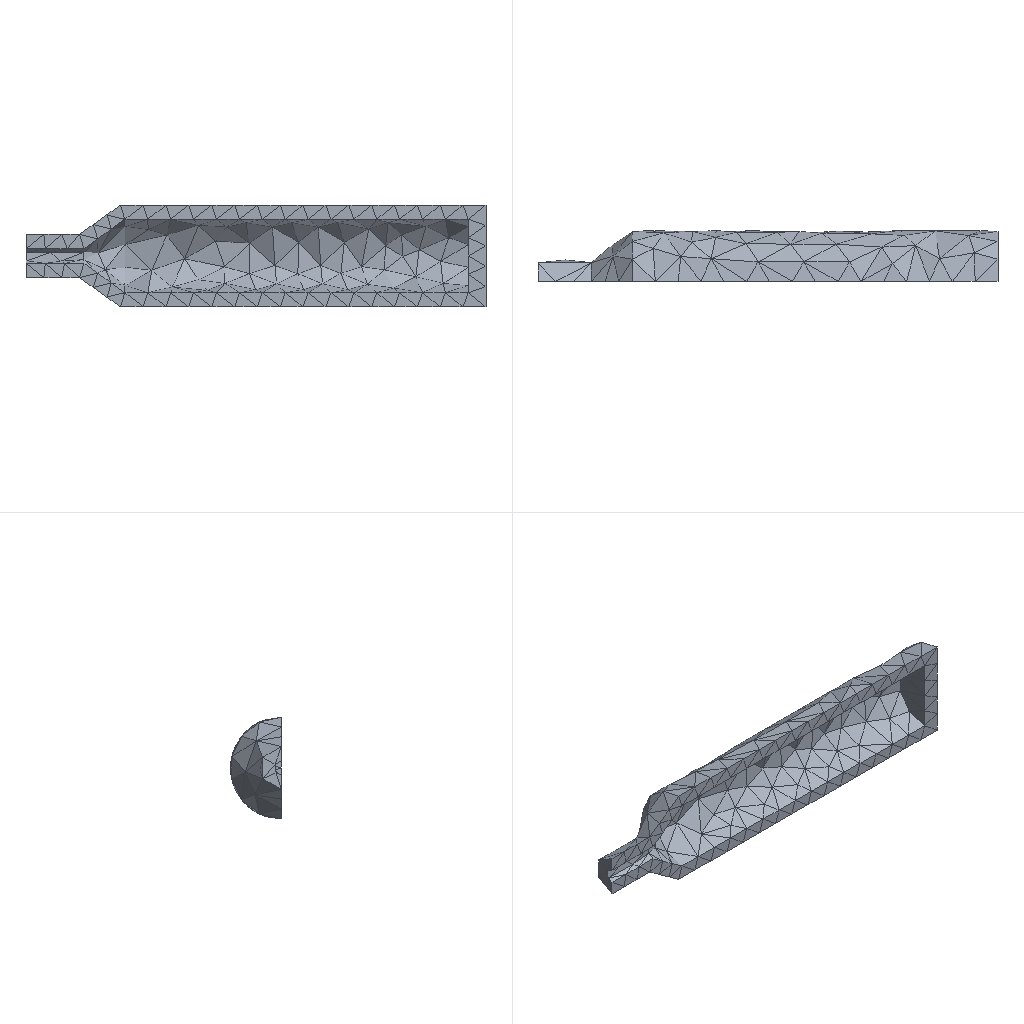Simulation study | ansys workbench
Ansys APDL input file, long lists of numbers shortened:
/batch
/config,noeldb,1     ! force off writing results to database
*get,_wallstrt,active,,time,wall
! ANSYS input file written by Workbench version 2022 R1
! File used for geometry attach:
/title,____--____ (B5)
! ****** Begin Custom Load Command Snippet ******
/COM, ACT Extensions:
/COM,     LSDYNA, 2021.1
/COM,
! ****** End   Custom Load Command Snippet ******
*DIM,_wb_ProjectScratch_dir,string,248
_wb_ProjectScratch_dir(1) = ''
*DIM,_wb_SolverFiles_dir,string,248
_wb_SolverFiles_dir(1) = ''
*DIM,_wb_userfiles_dir,string,248
_wb_userfiles_dir(1) = ''
/com,--- Data in consistent NMM units. See Solving Units in the help system for more information.
/units,MPA
/nopr
/wb,file,start              !  signify a WB generated input file
/prep7
! Turn off shape checking because checks already performed inside WB mesher.
! See help system for more information.
SHPP,OFF,,NOWARN
/nolist
etcon,set             ! allow ANSYS to choose best KEYOP's for 180x elements, resets any applicable keyopt to MAPDL defaults
/com,*********** Nodes for the whole assembly ***********
nblock,3,,1436
(1i9,3e20.9e3)
        1     1.304000000E+03     0.000000000E+00    -1.443258926E+02
! (1305 more lines like these left out)
-1
/wb,elem,start            !  set before creation of elements
/com,*********** Elements for Body 1 "__2-FreeParts|__-__2" ***********
et,1,187
eblock,19,solid,,578
(19i9)
        1        1        1        1        0        0        0        0       10        0        1      158      227      228      222     1034     1276     1035     1032
! (1155 more lines like these left out)
-1
/wb,elem,end               !  done creating elements
/com,*********** Send User Defined Coordinate System(s) ***********
csys,0
toffst,273.15,  ! Temperature offset from absolute zero
/com,*********** Set Reference Temperature ***********
tref,22.
/wb,mat,start              !  starting to send materials
/com,*********** Send Materials ***********
Temperature = 'TEMP' ! Temperature
MP,DENS,1,7.85e-09,	! tonne mm^-3
MP,ALPX,1,1.2e-05,	! C^-1
MP,C,1,434000000,	! mm^2 s^-2 C^-1
MP,KXX,1,60.5,	! tonne mm s^-3 C^-1
MP,RSVX,1,0.00017,	! ohm mm
MP,EX,1,200000,	! tonne s^-2 mm^-1
MP,NUXY,1,0.3,
MP,MURX,1,10000,
/wb,mat,end                !  done sending materials
!************************* Model Summary ********************
!__2-FreeParts|__-__2,	结构钢,	matid,	1
!************************* End Model Summary ********************
! get the diagonal of the bounding box. Needed later for other things
*get,_xmin,node,,mnloc,x
*get,_ymin,node,,mnloc,y
*get,_zmin,node,,mnloc,z
*get,_xmax,node,,mxloc,x
*get,_ymax,node,,mxloc,y
*get,_zmax,node,,mxloc,z
_ASMDIAG=(_xmax-_xmin)*(_xmax-_xmin)+(_ymax-_ymin)*(_ymax-_ymin)+(_zmax-_zmin)*(_zmax-_zmin)
_ASMDIAG=SQRT(_ASMDIAG)
/wb,contact,start          !  starting to send contact
/wb,contact,end            !  done creating contacts
/golist
/wb,load,start             !  starting to send loads
/com,*********** Fixed Supports ***********
CMBLOCK,_FIXEDSU,NODE,      325
(8i10)
         1         2         3         4         5         6         7         8
! (40 more lines like these left out)
cmsel,s,_FIXEDSU
d,all,all
nsel,all
/com,*********** Define Pressure Using Surface Effect Elements "__" ***********
et,2,154
eblock,10,,,128
(15i9)
     1061        2        2        2        0       79       81      122      122      638      646      122      640
! (127 more lines like these left out)
-1
esel,s,type,,2
keyop,2,7,0                ! Use deformed area for application of load
esel,all
/com,*********** Define Pressure Using Surface Effect Elements "__ 2" ***********
et,3,154
eblock,10,,,174
(15i9)
     1189        3        3        3        0        7        8      179      179      280      288      179      284
! (173 more lines like these left out)
-1
esel,s,type,,3
keyop,3,7,0                ! Use deformed area for application of load
esel,all
esel,all
/gst,on,on
fini
*get,_numnode,node,0,count
*get,_numelem,elem,0,count
*get, _MAXELEMNUM, elem, 0, NUM, MAX
*get, _MAXNODENUM, node, 0, NUM, MAX
*get, _MAXELEMTYPE, etyp, 0, NUM, MAX
*get, _MAXREALCONST, real, 0, NUM, MAX
/go
/wb,load,end               !  done creating loads
/com,--- Number of total nodes = %_numnode%
/com,--- Number of contact elements = 302
/com,--- Number of spring elements = 0
/com,--- Number of bearing elements = 0
/com,--- Number of solid elements = 578
/com,--- Number of condensed parts = 0
/com,--- Number of total elements = %_numelem%
*get,_wallbsol,active,,time,wall
/com,****************************************************************************
/com,*************************    SOLUTION       ********************************
/com,****************************************************************************
/solu
antype,0                   ! static analysis
_thickRatio=  0     ! Ratio of thick parts in the model
eqsl,sparse,,,,,1
cntr,print,1               ! print out contact info and also make no initial contact an error
dmpoption,emat,no             ! Don't combine emat file for DANSYS
dmpoption,esav,no             ! Don't combine esav file for DANSYS
nldiag,cont,iter           ! print out contact info each equilibrium iteration
rescontrol,,none                 ! Do not keep any restart files
/com,****************************************************
/com,******************* SOLVE FOR LS 1 OF 1 ****************
esel,s,type,,2
nsle
sf,all,pres,60.
esel,s,type,,3
nsle
sf,all,pres,20.
nsel,all
esel,all
esel,all
/nopr
/gopr
nsub,1,1,1
time,1.
outres,erase
outres,all,none
outres,nsol,all,
outres,rsol,all
outres,eangl,all
outres,etmp,all
outres,veng,all
outres,strs,all,
outres,epel,all,
outres,eppl,all,
outres,cont,all,
! *********** WB SOLVE COMMAND ***********
! check interactive state
*get,ANSINTER_,active,,int
*if,ANSINTER_,ne,0,then
/eof
*endif
solve
/com *************** Write FE CONNECTORS *********
CEWRITE,file,ce,,INTE
/com,****************************************************
/com,*************** FINISHED SOLVE FOR LS 1 *************
*get,_wallasol,active,,time,wall
/nopr
*get,_numnode,node,0,count
*get,_numelem,elem,0,count
*get, _MAXELEMNUM, elem, 0, NUM, MAX
*get, _MAXNODENUM, node, 0, NUM, MAX,,,INTERNAL
*get, _MAXELEMTYPE, etyp, 0, NUM, MAX
*get, _MAXREALCONST, real, 0, NUM, MAX
/gopr
/post1
xmlo,ENCODING,ISO-8859-1
xmlo,parm
/xml,parm,xml
fini
/gopr
*get,_walldone,active,,time,wall
_preptime=(_wallbsol-_wallstrt)*3600
_solvtime=(_wallasol-_wallbsol)*3600
_posttime=(_walldone-_wallasol)*3600
_totaltim=(_walldone-_wallstrt)*3600
*get,_dlbratio,active,0,solu,dlbr
*get,_combtime,active,0,solu,comb
*get,_ssmode,active,0,solu,ssmm
*get,_ndofs,active,0,solu,ndof
*get,_sol_end_time,active,0,set,time
*if,_sol_end_time,eq,1.,then
/fclean				!clean distributed files
*endif
/com,--- Total number of nodes = %_numnode%
/com,--- Total number of elements = %_numelem%
/com,--- Element load balance ratio = %_dlbratio%
/com,--- Time to combine distributed files = %_combtime%
/com,--- Sparse memory mode = %_ssmode%
/com,--- Number of DOF = %_ndofs%
/wb,file,end               ! done with WB generated input